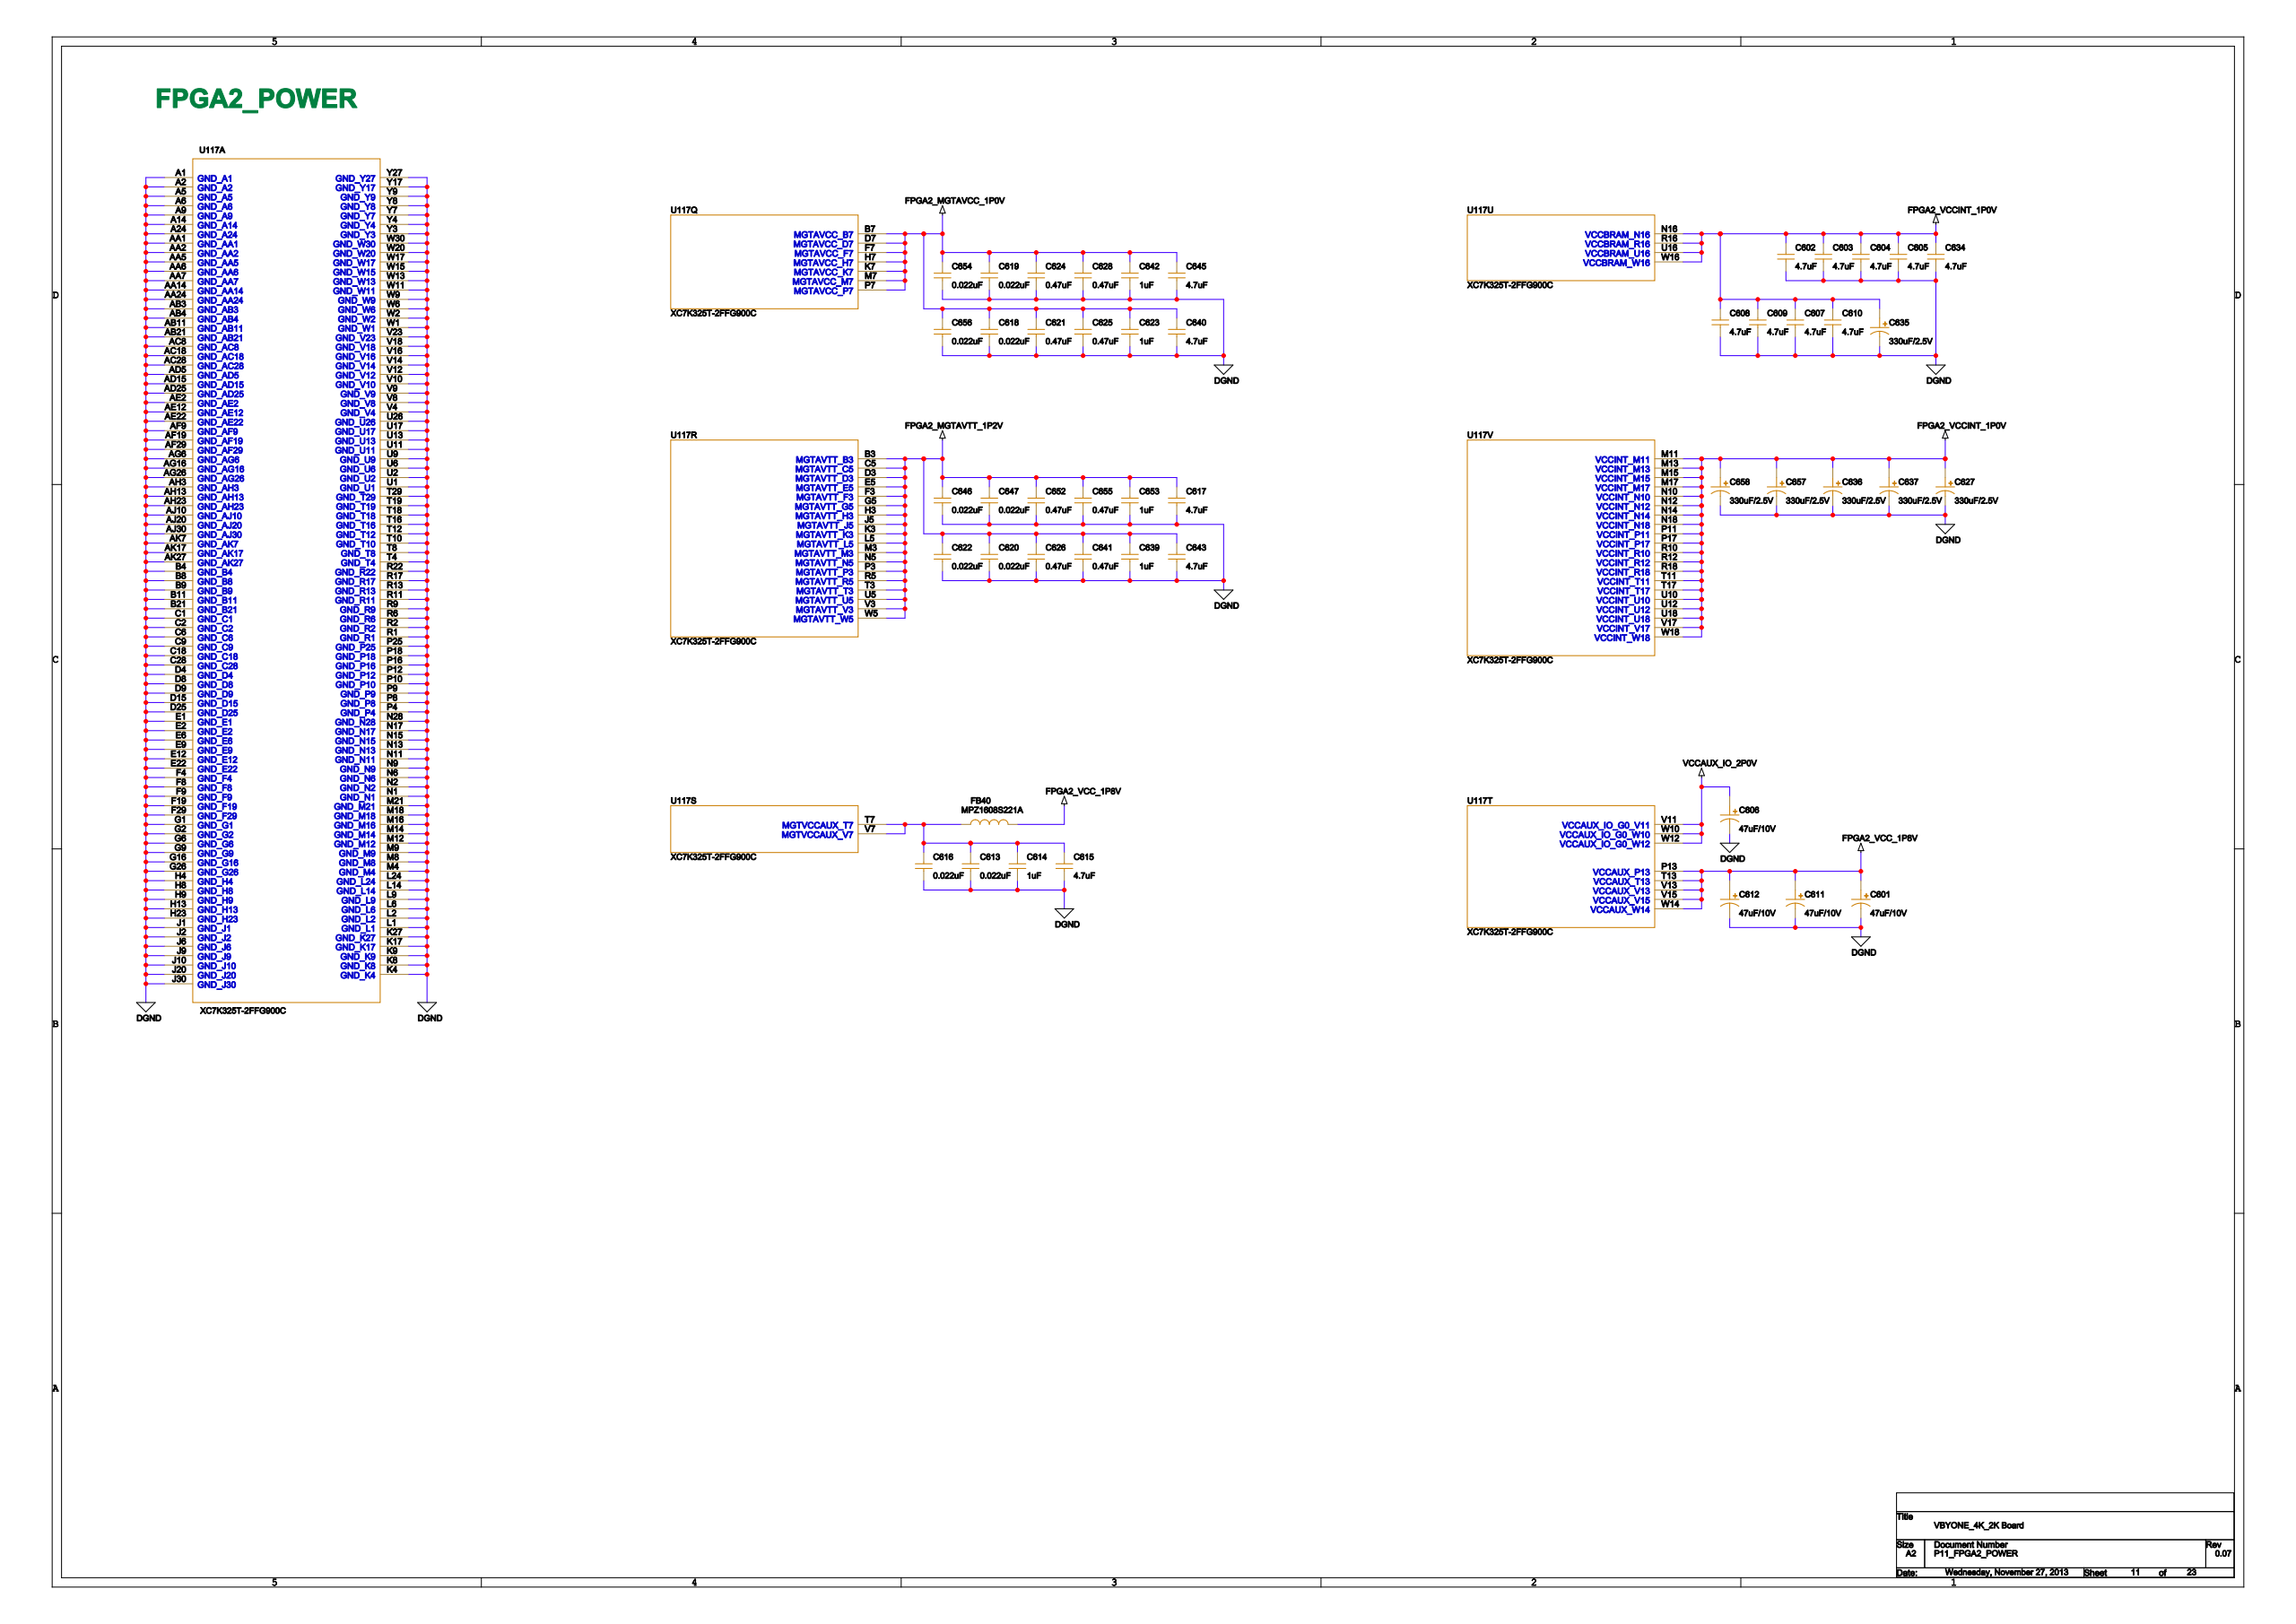Circuit board | Cadence Allegro | 1712 parts | 1495 nets | one sheet of the schematic
Parts on this sheet (reference | value | footprint):
C601 | 47uF/10V | CEC3528RZAS
C602 | 4.7uF | CRC1608RZAS
C603 | 4.7uF | CRC1608RZAS
C604 | 4.7uF | CRC1608RZAS
C605 | 4.7uF | CRC1608RZAS
C606 | 47uF/10V | CEC3528RZAS
C607 | 4.7uF | CRC1608RZAS
C608 | 4.7uF | CRC1608RZAS
C609 | 4.7uF | CRC1608RZAS
C610 | 4.7uF | CRC1608RZAS
C611 | 47uF/10V | CEC3528RZAS
C612 | 47uF/10V | CEC3528RZAS
C613 | 0.022uF | CRC1005RZAS
C614 | 1uF | CRC1608RZAS
C615 | 4.7uF | CRC1608RZAS
C616 | 0.022uF | CRC1005RZAS
C617 | 4.7uF | CRC1608RZAS
C618 | 0.022uF | CRC1005RZAS
C619 | 0.022uF | CRC1005RZAS
C620 | 0.022uF | CRC1005RZAS
C621 | 0.47uF | CRC1608RZAS
C622 | 0.022uF | CRC1005RZAS
C623 | 1uF | CRC1608RZAS
C624 | 0.47uF | CRC1608RZAS
C625 | 0.47uF | CRC1608RZAS
C626 | 0.47uF | CRC1608RZAS
C627 | 330uF/2.5V | CEC3528RZAS
C628 | 0.47uF | CRC1608RZAS
C634 | 4.7uF | CRC1608RZAS
C635 | 330uF/2.5V | CEC3528RZAS
C636 | 330uF/2.5V | CEC3528RZAS
C637 | 330uF/2.5V | CEC3528RZAS
C639 | 1uF | CRC1608RZAS
C640 | 4.7uF | CRC1608RZAS
C641 | 0.47uF | CRC1608RZAS
C642 | 1uF | CRC1608RZAS
C643 | 4.7uF | CRC1608RZAS
C645 | 4.7uF | CRC1608RZAS
C646 | 0.022uF | CRC1005RZAS
C647 | 0.022uF | CRC1005RZAS
C652 | 0.47uF | CRC1608RZAS
C653 | 1uF | CRC1608RZAS
C654 | 0.022uF | CRC1005RZAS
C655 | 0.47uF | CRC1608RZAS
C656 | 0.022uF | CRC1005RZAS
C657 | 330uF/2.5V | CEC3528RZAS
C658 | 330uF/2.5V | CEC3528RZAS
FB40 | MPZ1608S221A | LSC1608RZAS
U9 | SII1161CTU | QFP100RCBS
U10 | SII1161CTU | QFP100RCBS
U16 | SII1161CTU | QFP100RCBS
U26 | K4B4G1646B-HCK0 | BGA096RFDS
U117 | XC7K325T-2FFG900C | BGA900RGAS
Nets of these parts (net: part-pin ...):
DGND: C601-2 C602-2 C603-2 C604-2 C605-2 C606-2 C607-2 C608-2 C609-2 C610-2 C611-2 C612-2 C613-2 C614-2 C615-2 C616-2 C617-2 C618-2 C619-2 C620-2 C621-2 C622-2 C623-2 C624-2 C625-2 C626-2 C627-2 C628-2 C634-2 C635-2 C636-2 C637-2 C639-2 C640-2 C641-2 C642-2 C643-2 C645-2 C646-2 C647-2 C652-2 C653-2 C654-2 C655-2 C656-2 C657-2 C658-2 U9-5 U10-5 U16-5 U26-A9 U26-B3 U26-B9 U26-D8 U26-E1 U26-E2 U26-F9 U26-G1 U26-G9 U26-J2 U26-M9 U26-P9 U117-A1 U117-A2 U117-A5 U117-A6 U117-A9 U117-A14 U117-A24 U117-AA1 U117-AA2 U117-AA5 U117-AA6 U117-AA7 U117-AA14 U117-AA24 U117-AB3 U117-AB4 U117-AB11 U117-AB21 U117-AC8 U117-AC18 U117-AC28 U117-AD5 U117-AD15 U117-AD25 U117-AE2 U117-AE12 U117-AE22 U117-AF9 U117-AF19 U117-AF29 U117-AG6 U117-AG16 U117-AG26 U117-AH3 U117-AH13 U117-AH23 U117-AJ10 U117-AJ20 U117-AJ30 U117-AK7 U117-AK17 U117-AK27 U117-B4 U117-B8 U117-B9 U117-B11 U117-B21 U117-C1 U117-C2 U117-C6 U117-C9 U117-C18 U117-C28 U117-D4 U117-D8 U117-D9 U117-D15 U117-D25 U117-E1 U117-E2 U117-E6 U117-E9 U117-E12 U117-E22 U117-F4 U117-F8 U117-F9 U117-F19 U117-F29 U117-G1 U117-G2 U117-G6 U117-G9 U117-G16 U117-G26 U117-H4 U117-H8 U117-H9 U117-H13 U117-H23 U117-J1 U117-J2 U117-J6 U117-J9 U117-J10 U117-J20 U117-J30 U117-K4 U117-K8 U117-K9 U117-K17 U117-K27 U117-L1 U117-L2 U117-L6 U117-L9 U117-L14 U117-L24 U117-M4 U117-M8 U117-M9 U117-M12 U117-M14 U117-M16 U117-M18 U117-M21 U117-N1 U117-N2 U117-N6 U117-N9 U117-N11 U117-N13 U117-N15 U117-N17 U117-N28 U117-P4 U117-P8 U117-P9 U117-P10 U117-P12 U117-P16 U117-P18 U117-P25 U117-R1 U117-R2 U117-R6 U117-R9 U117-R11 U117-R13 U117-R17 U117-R22 U117-T4 U117-T8 U117-T10 U117-T12 U117-T16 U117-T18 U117-T19 U117-T29 U117-U1 U117-U2 U117-U6 U117-U9 U117-U11 U117-U13 U117-U17 U117-U26 U117-V4 U117-V8 U117-V9 U117-V10 U117-V12 U117-V14 U117-V16 U117-V18 U117-V23 U117-W1 U117-W2 U117-W6 U117-W9 U117-W11 U117-W13 U117-W15 U117-W17 U117-W20 U117-W30 U117-Y3 U117-Y4 U117-Y7 U117-Y8 U117-Y9 U117-Y17 U117-Y27
FPGA2_VCC_1P8V: C601-1 C611-1 C612-1 FB40-2 U117-P13 U117-T13 U117-V13 U117-V15 U117-W14
FPGA2_VCCINT_1P0V: C602-1 C603-1 C604-1 C605-1 C607-1 C608-1 C609-1 C610-1 C627-1 C634-1 C635-1 C636-1 C637-1 C657-1 C658-1 U117-M11 U117-M13 U117-M15 U117-M17 U117-N10 U117-N12 U117-N14 U117-N16 U117-N18 U117-P11 U117-P17 U117-R10 U117-R12 U117-R16 U117-R18 U117-T11 U117-T17 U117-U10 U117-U12 U117-U16 U117-U18 U117-V17 U117-W16 U117-W18
FPGA2_MGTAVTT_1P2V: C617-1 C620-1 C622-1 C626-1 C639-1 C641-1 C643-1 C646-1 C647-1 C652-1 C653-1 C655-1 U117-B3 U117-C5 U117-D3 U117-E5 U117-F3 U117-G5 U117-H3 U117-J5 U117-K3 U117-L5 U117-M3 U117-N5 U117-P3 U117-R5 U117-T3 U117-U5 U117-V3 U117-W5
FPGA2_MGTAVCC_1P0V: C618-1 C619-1 C621-1 C623-1 C624-1 C625-1 C628-1 C640-1 C642-1 C645-1 C654-1 C656-1 U117-B7 U117-D7 U117-F7 U117-H7 U117-K7 U117-M7 U117-P7
VCCAUX_IO_2P0V: C606-1 U117-V11 U117-W10 U117-W12
N18862133: C613-1 C614-1 C615-1 C616-1 FB40-1 U117-T7 U117-V7